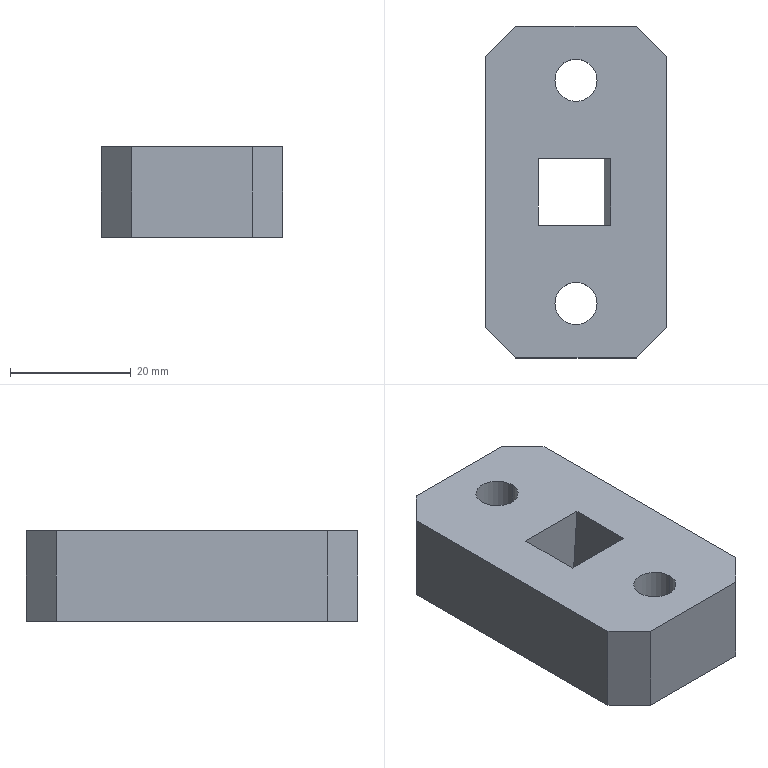Part | Creo | 1 solid | 150 faces | box 30.003 x 55 x 15 mm | volume 20068 mm3 | other 91 | plane 48 | cylinder 11 | commonest cylinder face diameters 7 x4 11 x4 1.421 x2 22.406 x1